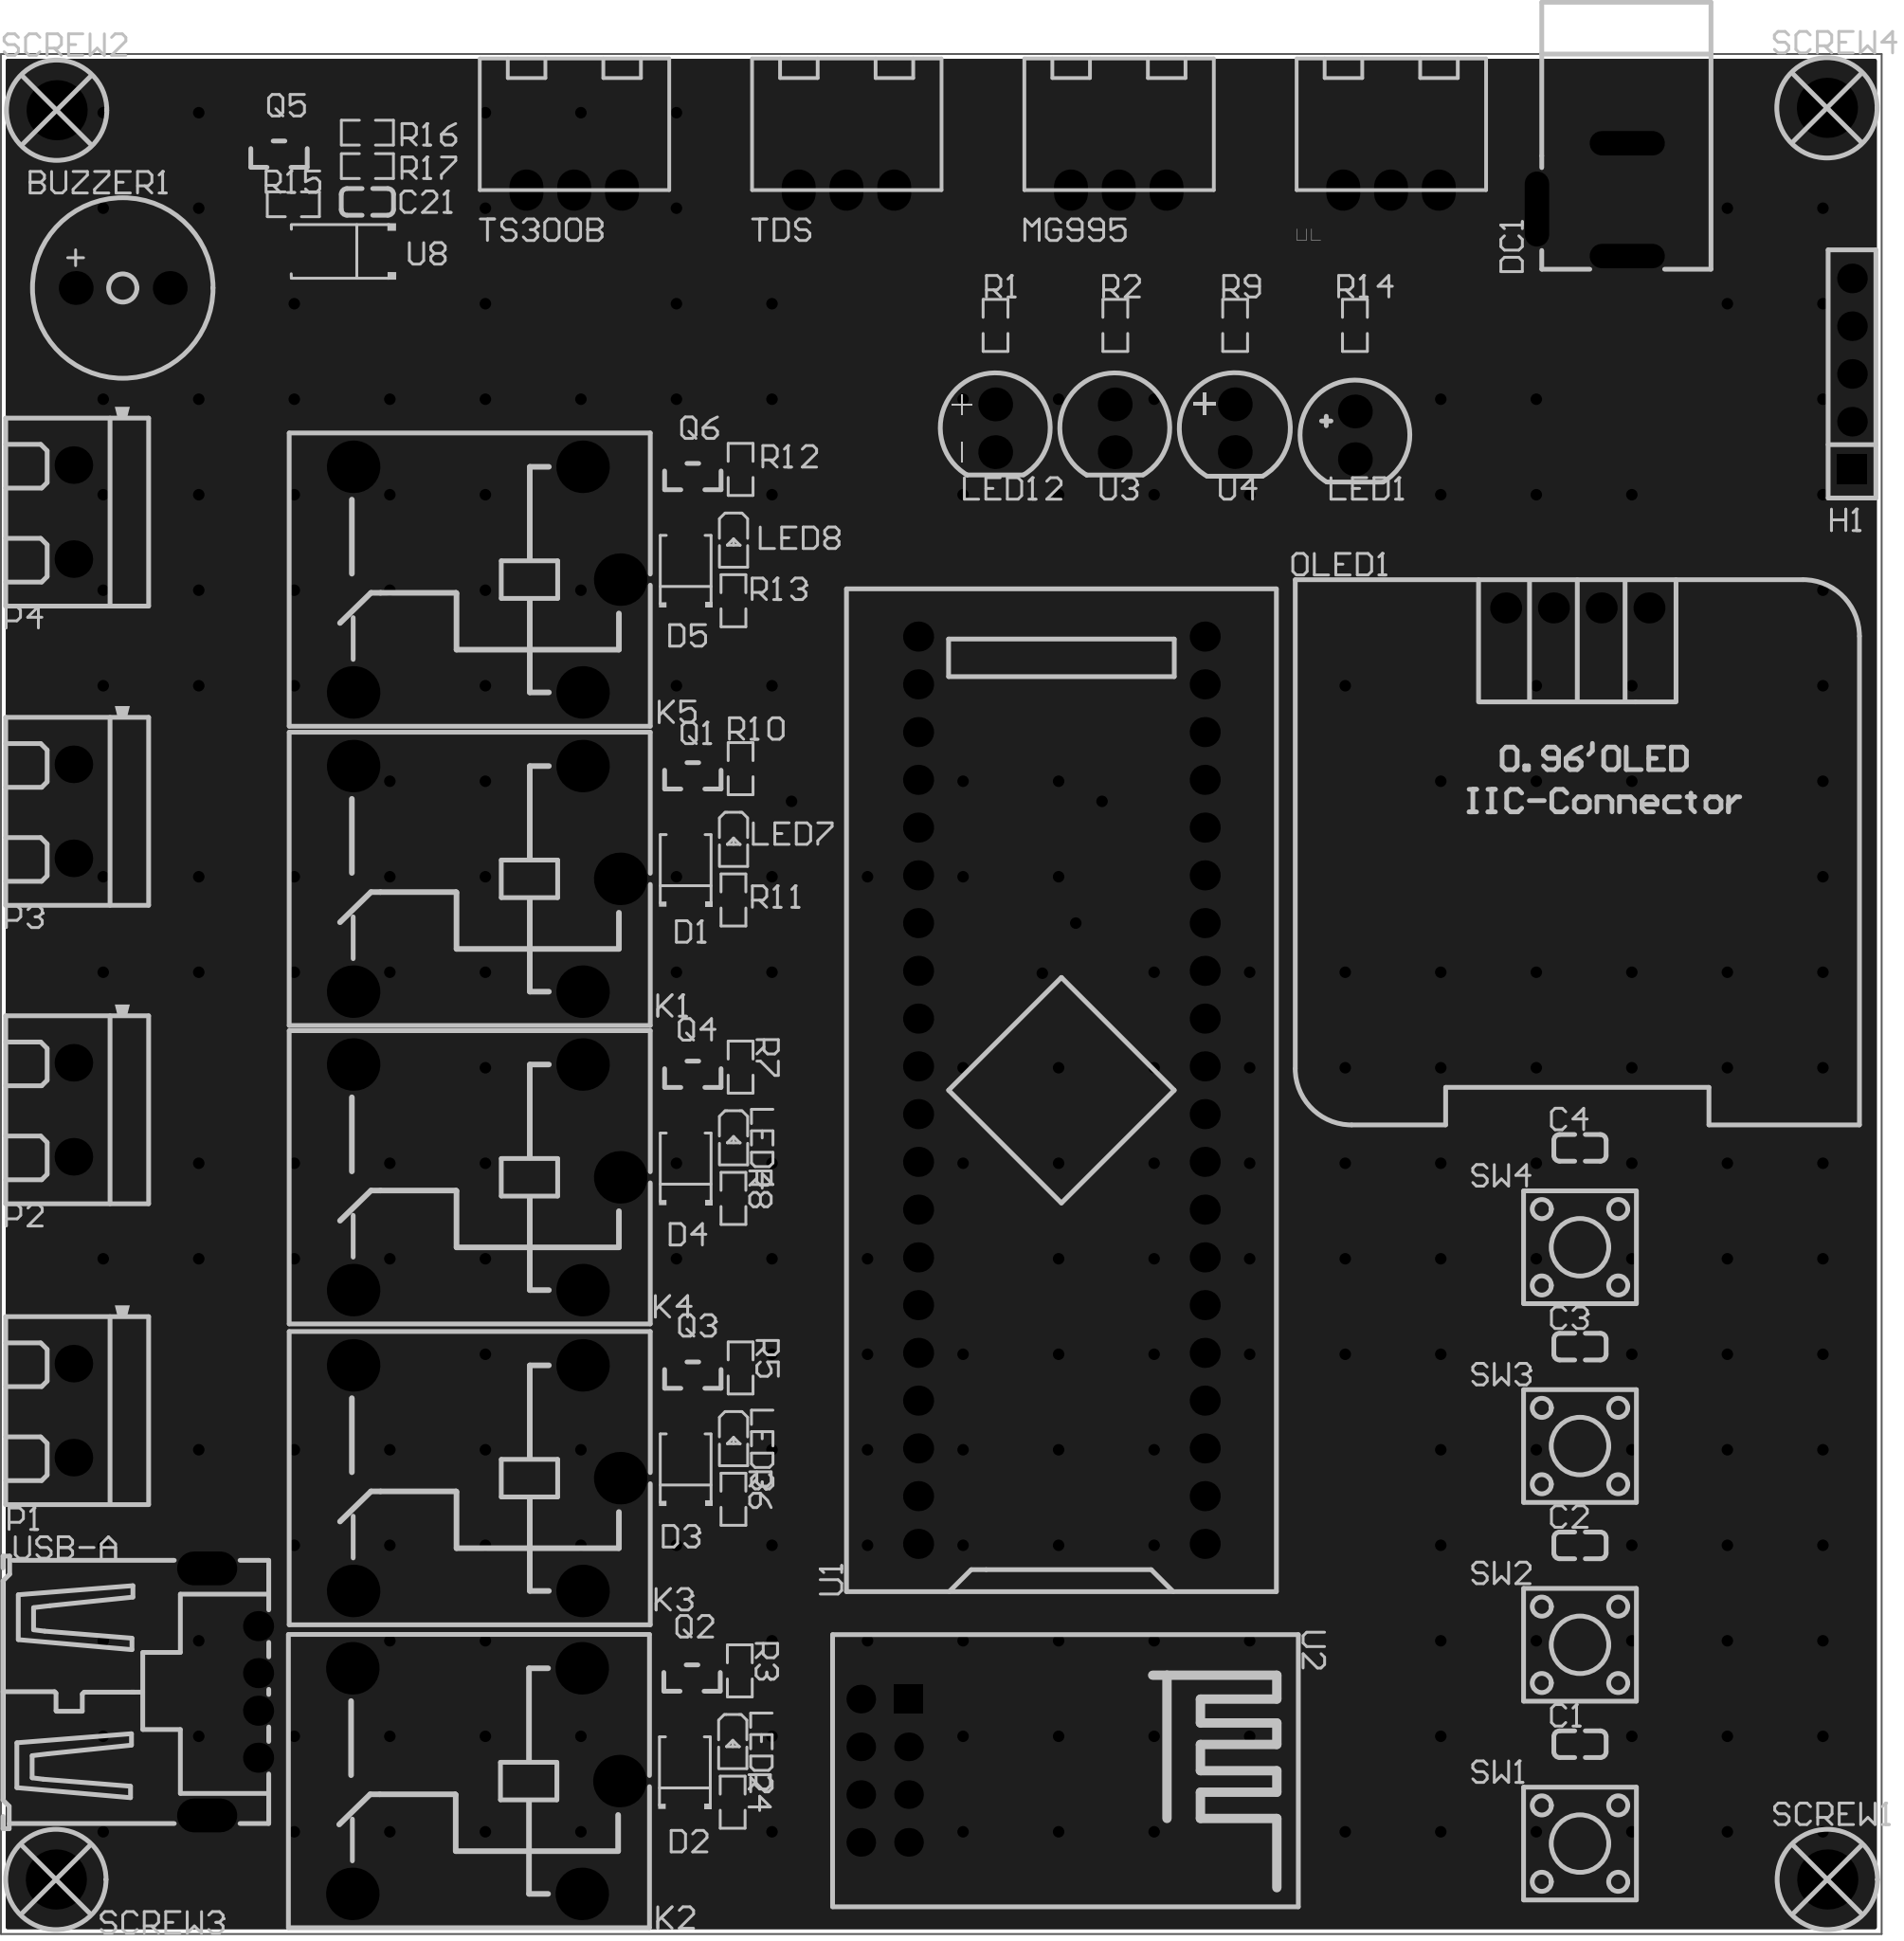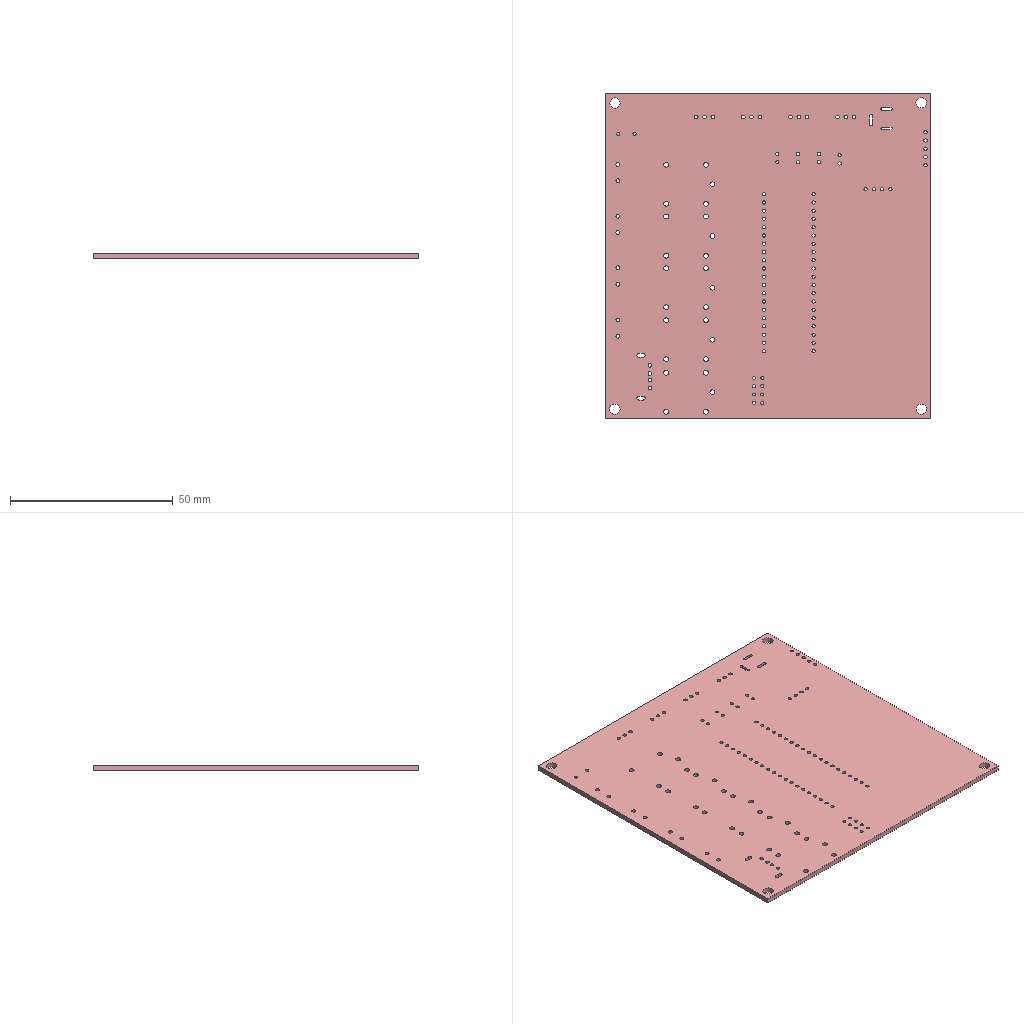Circuit board layout | Altium Designer | box 100 x 100 x 1.6 mm
Layer stack:
# Altium Designer layer stack of  (unit mm; dielectric type: 0 none, 1 core, 2 prepreg, 3 surface material)
index,name,kind,layer,copper_thickness_mm,dielectric_type,dielectric_thickness_mm,dielectric_material,dielectric_constant
0,Top Paste Mask Layer,other,,,,,,
1,Top Silkscreen Layer,other,,,,,,
2,Top Solder Mask Layer,dielectric,,,3,0.01,,3.3
3,Top Layer,copper,Top Layer,0.035,,,,
4,Dielectric1,dielectric,,,3,1.51,FR4,4.5
5,Bottom Layer,copper,Bottom Layer,0.035,,,,
6,Bottom Solder Mask Layer,dielectric,,,3,0.01,,3.3
7,Bottom Silkscreen Layer,other,,,,,,
8,Bottom Paste Mask Layer,other,,,,,,
# drill layer pairs: low layer,high layer
drill_pair,Top Layer,Bottom Layer
Part placement:
Designator,Comment,Layer,Footprint,Center-X(mm),Center-Y(mm),Rotation
C1,100nF,TopLayer,C0603,170.194,90.565,0
C2,100nF,TopLayer,C0603,170.194,101.138,0
C3,100nF,TopLayer,C0603,170.194,111.711,0
C4,100nF,TopLayer,C0603,170.194,122.284,0
C21,100nF,TopLayer,C0603,105.718,172.6,0
D1,M7F,TopLayer,SMAF_L3.5-W2.6-LS4.7-RD,122.641,137.12,90
D2,M7F,TopLayer,SMAF_L3.5-W2.6-LS4.7-RD,122.599,89.13,90
D3,M7F,TopLayer,SMAF_L3.5-W2.6-LS4.7-RD,122.641,105.243,90
D4,M7F,TopLayer,SMAF_L3.5-W2.6-LS4.7-RD,122.641,121.245,90
D5,M7F,TopLayer,SMAF_L3.5-W2.6-LS4.7-RD,122.641,153.037,90
H1,,TopLayer,HDR-TH_5P-P2.54-V-F,184.658,163.449,90
K1,SRD-DC5V-SL-C,TopLayer,RELAY-TH_SRD-DCXXV-SL-C,112.06,136.593,180
K2,SRD-DC5V-SL-C,TopLayer,RELAY-TH_SRD-DCXXV-SL-C,112.018,88.603,180
K3,SRD-DC5V-SL-C,TopLayer,RELAY-TH_SRD-DCXXV-SL-C,112.06,104.716,180
K4,SRD-DC5V-SL-C,TopLayer,RELAY-TH_SRD-DCXXV-SL-C,112.06,120.718,180
K5,SRD-DC5V-SL-C,TopLayer,RELAY-TH_SRD-DCXXV-SL-C,112.06,152.509,180
LED1,blue,TopLayer,LED-TH_BD5.9-P2.54-RD_BLUE,158.227,160.184,90
LED2,MS-PTV1608NWAF-B02,TopLayer,LED0603-RD,125.139,90.654,270
LED3,MS-PTV1608NWAF-B02,TopLayer,LED0603-RD,125.181,106.767,270
LED4,MS-PTV1608NWAF-B02,TopLayer,LED0603-RD,125.181,122.769,270
LED7,MS-PTV1608NWAF-B02,TopLayer,LED0603-RD,125.181,138.644,270
LED8,MS-PTV1608NWAF-B02,TopLayer,LED0603-RD,125.181,154.561,270
LED12,red,TopLayer,LED-TH_BD5.9-P2.54-RD_RED,139.1,160.56,90
MG995,,TopLayer,XH2.54-3P,145.669,173.228,0
OLED1,,TopLayer,0.96OLED_4P,170.053,151.003,0
P1,KF301-2P terminal block,TopLayer,CONN-TH_XY301V-A-5.0-2P,90.087,108.307,90
P2,KF301-2P terminal block,TopLayer,CONN-TH_XY301V-A-5.0-2P,90.087,124.309,90
P3,KF301-2P terminal block,TopLayer,CONN-TH_XY301V-A-5.0-2P,90.087,140.184,90
P4,KF301-2P terminal block,TopLayer,CONN-TH_XY301V-A-5.0-2P,90.087,156.101,90
Q1,,TopLayer,S8050_SOT-23,123.022,142.073,90
Q2,,TopLayer,S8050_SOT-23,122.98,94.083,90
Q3,,TopLayer,S8050_SOT-23,123.022,110.196,90
Q4,,TopLayer,S8050_SOT-23,123.022,126.198,90
Q5,,TopLayer,S8050_SOT-23,101.019,175.14,90
Q6,,TopLayer,S8050_SOT-23,123.022,157.99,90
R1,1K,TopLayer,R0603,139.117,166.031,270
R2,1K,TopLayer,R0603,145.487,166.031,270
R3,330,TopLayer,R0603,125.52,94.464,270
R4,1K,TopLayer,R0603,125.139,87.479,270
R5,330,TopLayer,R0603,125.562,110.577,270
R6,1K,TopLayer,R0603,125.181,103.592,270
R7,330,TopLayer,R0603,125.562,126.579,270
R8,1K,TopLayer,R0603,125.181,119.594,270
R9,1K,TopLayer,R0603,151.857,166.031,270
R10,330,TopLayer,R0603,125.562,142.454,270
R11,1K,TopLayer,R0603,125.181,135.469,270
R12,330,TopLayer,R0603,125.562,158.371,270
R13,1K,TopLayer,R0603,125.181,151.386,270
R14,1K,TopLayer,R0603,158.227,166.031,270
R15,0R,TopLayer,R0603,101.781,172.473,0
R16,1K,TopLayer,R0603,105.718,176.283,0
R17,4.7K,TopLayer,R0603,105.718,174.505,0
SCREW1,,TopLayer,M3螺丝,183.344,83.37,0
SCREW2,,TopLayer,M3螺丝,89.194,177.476,0
SCREW3,,TopLayer,M3螺丝,89.154,83.37,0
SCREW4,,TopLayer,M3螺丝,183.325,177.603,0
SW1,,TopLayer,SW-SMD_4P-L6.0-W6.0-P4.50-LS9.0-2,170.194,85.278,0
SW2,,TopLayer,SW-SMD_4P-L6.0-W6.0-P4.50-LS9.0-2,170.194,95.851,0
SW3,,TopLayer,SW-SMD_4P-L6.0-W6.0-P4.50-LS9.0-2,170.194,106.424,0
SW4,,TopLayer,SW-SMD_4P-L6.0-W6.0-P4.50-LS9.0-2,170.194,116.997,0
TDS,,TopLayer,XH2.54-3P,131.191,173.228,0
TS300B,,TopLayer,XH2.54-3P,116.713,173.228,0
U1,LCKFB-DKX-STM32F103C8T6,TopLayer,CONN-TH_L53.3-W22.9_STM32F103C8T6-CARD,142.621,125.349,90
U2,ESP8266-01S,TopLayer,WIFIM-TH_ESP8266-01S,133.223,89.154,270
U3,green,TopLayer,LED-TH_BD5.9-P2.54-RD_GREEN,145.456,160.557,90
U4,yellow,TopLayer,LED-TH_BD5.9-P2.54-RD_YELLOW,151.84,160.563,90
U8,SS24-MS,TopLayer,SMA_L4.3-W2.6-LS5.1-RD,104.27,169.966,180
USB-A,USB-AF,TopLayer,USB-A-TH_USB-302-T,98.552,93.345,270
水温,,TopLayer,XH2.54-3P,160.147,173.228,0
BUZZER1,3kHz,TopLayer,BUZ-TH_BD9.6-P5.00-D0.7-FD,92.71,168.021,0
DC1,,TopLayer,DC-2.0,170.307,172.72,90
Pad and via stacks:
# Altium Designer via and pad stacks of  (unit mm). Each distinct definition once, with the count of objects using it.
# via: kind,start_layer,end_layer,hole_mm,diameter_mm,mode(0 simple;1 top-mid-bottom;2 full stack),diameter_per_layer,count,example_net
# pad: kind,layer,hole_mm,hole_type(0 round;1 square;2 slot),plating,top_size,top_shape(1 round;2 rect;3 octagon;9 rounded rect),mid_size,bottom_size,mode,footprint,size_per_layer,count,example
pad,Top Layer,0,0,plated,0.8x0.9,2,0.8x0.9,0.8x0.9,0,C0603,,10,C1.2
pad,Top Layer,0,0,plated,1.6x1.7,2,1.6x1.7,1.6x1.7,0,SMAF_L3.5-W2.6-LS4.7-RD,,10,D1.2
pad,Top Layer,0,0,plated,0.8x0.8,2,0.8x0.8,0.8x0.8,0,LED0603-RD,,10,LED2.2
pad,Top Layer,0,0,plated,1x0.8,2,1x0.8,1x0.8,0,S8050_SOT-23,,18,Q1.2
pad,Top Layer,0,0,plated,0.8065x0.864,2,0.8065x0.864,0.8065x0.864,0,R0603,,34,R1.2
pad,Top Layer,0,0,plated,2.3x1.5,2,2.3x1.5,2.3x1.5,0,SW-SMD_4P-L6.0-W6.0-P4.50-LS9.0-2,,16,SW1.1
pad,Top Layer,0,0,plated,2x2,2,2x2,2x2,0,SMA_L4.3-W2.6-LS5.1-RD,,2,U8.1
pad,Multi-Layer,1.02,0,plated,1.575x1.575,1,1.575x1.575,1.575x1.575,0,HDR-TH_5P-P2.54-V-F,,4,H1.5
pad,Multi-Layer,1.02,0,plated,1.575x1.575,2,1.575x1.575,1.575x1.575,0,HDR-TH_5P-P2.54-V-F,,1,H1.1
pad,Multi-Layer,1.524,0,plated,2.794x2.794,1,2.794x2.794,2.794x2.794,0,RELAY-TH_SRD-DCXXV-SL-C,,25,K1.2
pad,Multi-Layer,1,0,plated,1.8x1.8,1,1.8x1.8,1.8x1.8,0,LED-TH_BD5.9-P2.54-RD_BLUE,,2,LED1.1
pad,Multi-Layer,1,0,plated,1.8x1.8,1,1.8x1.8,1.8x1.8,0,LED-TH_BD5.9-P2.54-RD_RED,,2,LED12.2
pad,Multi-Layer,1.1,0,plated,1.8x2.2,1,1.8x2.2,1.8x2.2,0,XH2.54-3P,,12,MG995.3
pad,Multi-Layer,1,0,plated,1.65x1.65,1,1.65x1.65,1.65x1.65,0,0.96OLED_4P,,4,OLED1.4
pad,Multi-Layer,1.2,0,plated,2x2,1,2x2,2x2,0,CONN-TH_XY301V-A-5.0-2P,,8,P1.1
pad,Multi-Layer,3.2,0,plated,3.2x3.2,1,3.2x3.2,3.2x3.2,0,M3\u00C2\u00DD\u00CB\u00BF,,4,SCREW1.1
pad,Multi-Layer,1,0,plated,1.6x1.6,1,1.6x1.6,1.6x1.6,0,CONN-TH_L53.3-W22.9_STM32F103C8T6-CARD,,40,U1.1
pad,Multi-Layer,0.9144,0,plated,1.524x1.524,1,1.524x1.524,1.524x1.524,0,WIFIM-TH_ESP8266-01S,,7,U2.8
pad,Multi-Layer,0.9144,0,plated,1.524x1.524,2,1.524x1.524,1.524x1.524,0,WIFIM-TH_ESP8266-01S,,1,U2.1
pad,Multi-Layer,1,0,plated,1.8x1.8,1,1.8x1.8,1.8x1.8,0,LED-TH_BD5.9-P2.54-RD_GREEN,,2,U3.1
pad,Multi-Layer,1,0,plated,1.8x1.8,1,1.8x1.8,1.8x1.8,0,LED-TH_BD5.9-P2.54-RD_YELLOW,,2,U4.1
pad,Multi-Layer,1.1,0,plated,1.6x1.6,1,1.6x1.6,1.6x1.6,0,USB-A-TH_USB-302-T,,4,USB-A.1
pad,Multi-Layer,1.2,2,plated,3.2x1.8,1,3.2x1.8,3.2x1.8,0,USB-A-TH_USB-302-T,,2,USB-A.5
pad,Multi-Layer,1,0,plated,1.8x1.8,1,1.8x1.8,1.8x1.8,0,BUZ-TH_BD9.6-P5.00-D0.7-FD,,2,BUZZER1.2
pad,Multi-Layer,0.8001,2,plated,4x1.3,1,4x1.3,4x1.3,0,DC-2.0,,3,DC1.2
via,Top Layer,Bottom Layer,0.3048,0.61,0,,231,PA3
Copper pours:
name,layer,net,type(0 solid;1 hatched;2 none)
Bottom Layer-GND,Bottom Layer,GND,0
Top Layer-GND,Top Layer,GND,0
Design rules, without the lines most boards share:
# Altium Designer design rules of  (exported by Altium Designer, unit mm)
# columns: name | kind | enabled | priority | scope1 | scope2 | descriptor | typed fields (field=value)
creepage | 65 | enabled | 1 | All | All | Creepage Distance Constraint =(0mil) (All),(All) |